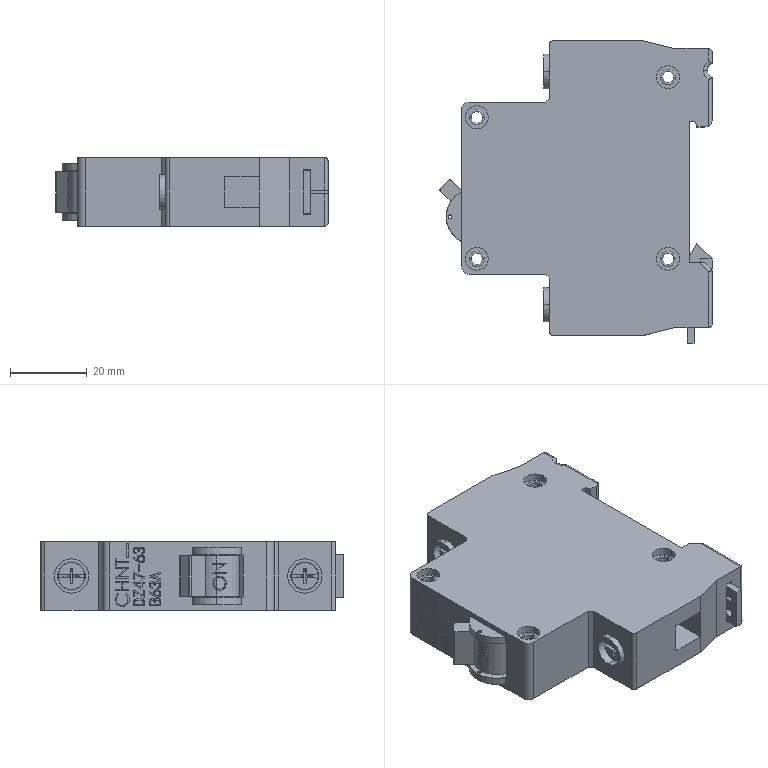Part | SolidWorks | features BaseBody 1 | 1 solid | 458 faces | box 71.146 x 79 x 18 mm | volume 70528 mm3 | plane 294 | cylinder 95 | spline 49 | torus 20 | commonest cylinder face diameters 4 x21 6 x16 2 x13 3 x8 1 x7 12 x7